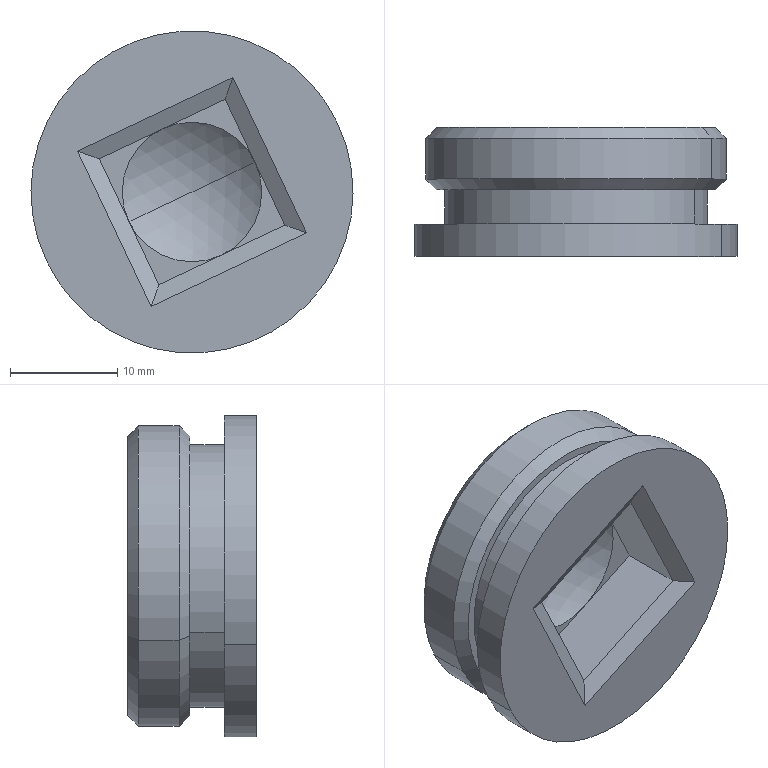Part | SolidWorks | features BaseBody 1 | 1 solid | 30 faces | box 30 x 12 x 30 mm | volume 5796 mm3 | plane 16 | cylinder 8 | cone 4 | sphere 2 | commonest cylinder face diameters 13 x2 24.5 x2 28 x2 30 x2
STEP:
#1=CARTESIAN_POINT('',(-57.117,-80.904,50.261));
#2=VERTEX_POINT('',#1);
#3=CARTESIAN_POINT('',(-31.809,-80.904,62.239));
#4=VERTEX_POINT('',#3);
#5=CARTESIAN_POINT('',(-44.463,-80.904,56.25));
#6=DIRECTION('',(0.,1.,0.));
#7=DIRECTION('',(0.9039,0.,0.4278));
#8=AXIS2_PLACEMENT_3D('',#5,#6,#7);
#9=CIRCLE('',#8,14.);
#10=EDGE_CURVE('',#2,#4,#9,.T.);
#11=ORIENTED_EDGE('',*,*,#10,.T.);
#12=CARTESIAN_POINT('',(-31.809,-77.104,62.239));
#13=VERTEX_POINT('',#12);
#14=CARTESIAN_POINT('',(-31.809,-81.904,62.239));
#15=DIRECTION('',(0.,1.,0.));
#16=VECTOR('',#15,1000.);
#17=LINE('',#14,#16);
#18=EDGE_CURVE('',#4,#13,#17,.T.);
#19=ORIENTED_EDGE('',*,*,#18,.T.);
#20=CARTESIAN_POINT('',(-57.117,-77.104,50.261));
#21=VERTEX_POINT('',#20);
#22=CARTESIAN_POINT('',(-44.463,-77.104,56.25));
#23=DIRECTION('',(0.,-1.,0.));
#24=DIRECTION('',(0.9039,0.,0.4278));
#25=AXIS2_PLACEMENT_3D('',#22,#23,#24);
#26=CIRCLE('',#25,14.);
#27=EDGE_CURVE('',#13,#21,#26,.T.);
#28=ORIENTED_EDGE('',*,*,#27,.T.);
#29=CARTESIAN_POINT('',(-57.117,-81.904,50.261));
#30=DIRECTION('',(0.,1.,0.));
#31=VECTOR('',#30,1000.);
#32=LINE('',#29,#31);
#33=EDGE_CURVE('',#2,#21,#32,.T.);
#34=ORIENTED_EDGE('',*,*,#33,.F.);
#35=EDGE_LOOP('',(#11,#19,#28,#34));
#36=FACE_OUTER_BOUND('',#35,.T.);
#37=CARTESIAN_POINT('',(-44.463,-81.904,56.25));
#38=DIRECTION('',(0.,1.,0.));
#39=DIRECTION('',(-0.9039,0.,-0.4278));
#40=AXIS2_PLACEMENT_3D('',#37,#38,#39);
#41=CYLINDRICAL_SURFACE('',#40,14.);
#42=ADVANCED_FACE('',(#36),#41,.T.);
#43=CARTESIAN_POINT('',(-33.39,-85.104,61.491));
#44=VERTEX_POINT('',#43);
#45=CARTESIAN_POINT('',(-55.535,-85.104,51.009));
#46=VERTEX_POINT('',#45);
#47=CARTESIAN_POINT('',(-44.463,-85.104,56.25));
#48=DIRECTION('',(0.,-1.,0.));
#49=DIRECTION('',(0.9039,0.,0.4278));
#50=AXIS2_PLACEMENT_3D('',#47,#48,#49);
#51=CIRCLE('',#50,12.25);
#52=EDGE_CURVE('',#44,#46,#51,.T.);
#53=ORIENTED_EDGE('',*,*,#52,.F.);
#54=CARTESIAN_POINT('',(-33.39,-81.904,61.491));
#55=VERTEX_POINT('',#54);
#56=CARTESIAN_POINT('',(-33.39,-85.104,61.491));
#57=DIRECTION('',(0.,1.,0.));
#58=VECTOR('',#57,1000.);
#59=LINE('',#56,#58);
#60=EDGE_CURVE('',#44,#55,#59,.T.);
#61=ORIENTED_EDGE('',*,*,#60,.T.);
#62=CARTESIAN_POINT('',(-55.535,-81.904,51.009));
#63=VERTEX_POINT('',#62);
#64=CARTESIAN_POINT('',(-44.463,-81.904,56.25));
#65=DIRECTION('',(0.,-1.,0.));
#66=DIRECTION('',(0.9039,0.,0.4278));
#67=AXIS2_PLACEMENT_3D('',#64,#65,#66);
#68=CIRCLE('',#67,12.25);
#69=EDGE_CURVE('',#55,#63,#68,.T.);
#70=ORIENTED_EDGE('',*,*,#69,.T.);
#71=CARTESIAN_POINT('',(-55.535,-85.104,51.009));
#72=DIRECTION('',(0.,1.,0.));
#73=VECTOR('',#72,1000.);
#74=LINE('',#71,#73);
#75=EDGE_CURVE('',#46,#63,#74,.T.);
#76=ORIENTED_EDGE('',*,*,#75,.F.);
#77=EDGE_LOOP('',(#53,#61,#70,#76));
#78=FACE_OUTER_BOUND('',#77,.T.);
#79=CARTESIAN_POINT('',(-44.463,-85.104,56.25));
#80=DIRECTION('',(0.,1.,0.));
#81=DIRECTION('',(-0.9039,0.,-0.4278));
#82=AXIS2_PLACEMENT_3D('',#79,#80,#81);
#83=CYLINDRICAL_SURFACE('',#82,12.25);
#84=ADVANCED_FACE('',(#78),#83,.T.);
#85=CARTESIAN_POINT('',(-30.905,-88.104,62.667));
#86=VERTEX_POINT('',#85);
#87=CARTESIAN_POINT('',(-58.021,-88.104,49.833));
#88=VERTEX_POINT('',#87);
#89=CARTESIAN_POINT('',(-44.463,-88.104,56.25));
#90=DIRECTION('',(0.,-1.,0.));
#91=DIRECTION('',(0.9039,0.,0.4278));
#92=AXIS2_PLACEMENT_3D('',#89,#90,#91);
#93=CIRCLE('',#92,15.);
#94=EDGE_CURVE('',#86,#88,#93,.T.);
#95=ORIENTED_EDGE('',*,*,#94,.F.);
#96=CARTESIAN_POINT('',(-30.905,-85.104,62.667));
#97=VERTEX_POINT('',#96);
#98=CARTESIAN_POINT('',(-30.905,-88.104,62.667));
#99=DIRECTION('',(0.,1.,0.));
#100=VECTOR('',#99,1000.);
#101=LINE('',#98,#100);
#102=EDGE_CURVE('',#86,#97,#101,.T.);
#103=ORIENTED_EDGE('',*,*,#102,.T.);
#104=CARTESIAN_POINT('',(-58.021,-85.104,49.833));
#105=VERTEX_POINT('',#104);
#106=CARTESIAN_POINT('',(-44.463,-85.104,56.25));
#107=DIRECTION('',(0.,-1.,0.));
#108=DIRECTION('',(0.9039,0.,0.4278));
#109=AXIS2_PLACEMENT_3D('',#106,#107,#108);
#110=CIRCLE('',#109,15.);
#111=EDGE_CURVE('',#97,#105,#110,.T.);
#112=ORIENTED_EDGE('',*,*,#111,.T.);
#113=CARTESIAN_POINT('',(-58.021,-88.104,49.833));
#114=DIRECTION('',(0.,1.,0.));
#115=VECTOR('',#114,1000.);
#116=LINE('',#113,#115);
#117=EDGE_CURVE('',#88,#105,#116,.T.);
#118=ORIENTED_EDGE('',*,*,#117,.F.);
#119=EDGE_LOOP('',(#95,#103,#112,#118));
#120=FACE_OUTER_BOUND('',#119,.T.);
#121=CARTESIAN_POINT('',(-44.463,-88.104,56.25));
#122=DIRECTION('',(0.,1.,0.));
#123=DIRECTION('',(-0.9039,0.,-0.4278));
#124=AXIS2_PLACEMENT_3D('',#121,#122,#123);
#125=CYLINDRICAL_SURFACE('',#124,15.);
#126=ADVANCED_FACE('',(#120),#125,.T.);
#127=CARTESIAN_POINT('',(-50.338,-81.504,53.469));
#128=VERTEX_POINT('',#127);
#129=CARTESIAN_POINT('',(-38.588,-81.504,59.031));
#130=VERTEX_POINT('',#129);
#131=CARTESIAN_POINT('',(-44.463,-81.504,56.25));
#132=DIRECTION('',(0.,1.,0.));
#133=DIRECTION('',(-0.9039,0.,-0.4278));
#134=AXIS2_PLACEMENT_3D('',#131,#132,#133);
#135=CIRCLE('',#134,6.5);
#136=EDGE_CURVE('',#128,#130,#135,.T.);
#137=ORIENTED_EDGE('',*,*,#136,.F.);
#138=CARTESIAN_POINT('',(-44.463,-79.104,56.25));
#139=VERTEX_POINT('',#138);
#140=CARTESIAN_POINT('',(-44.463,-89.104,56.25));
#141=DIRECTION('',(0.4278,0.,-0.9039));
#142=DIRECTION('',(-0.9039,0.,-0.4278));
#143=AXIS2_PLACEMENT_3D('',#140,#141,#142);
#144=CIRCLE('',#143,10.);
#145=EDGE_CURVE('',#128,#139,#144,.T.);
#146=ORIENTED_EDGE('',*,*,#145,.T.);
#147=CARTESIAN_POINT('',(-44.463,-89.104,56.25));
#148=DIRECTION('',(-0.4278,0.,0.9039));
#149=DIRECTION('',(0.9039,0.,0.4278));
#150=AXIS2_PLACEMENT_3D('',#147,#148,#149);
#151=CIRCLE('',#150,10.);
#152=EDGE_CURVE('',#130,#139,#151,.T.);
#153=ORIENTED_EDGE('',*,*,#152,.F.);
#154=EDGE_LOOP('',(#137,#146,#153));
#155=FACE_OUTER_BOUND('',#154,.T.);
#156=CARTESIAN_POINT('',(-44.463,-89.104,56.25));
#157=DIRECTION('',(0.4278,0.,-0.9039));
#158=DIRECTION('',(0.9039,0.,0.4278));
#159=AXIS2_PLACEMENT_3D('',#156,#157,#158);
#160=SPHERICAL_SURFACE('',#159,10.);
#161=ADVANCED_FACE('',(#155),#160,.F.);
#162=CARTESIAN_POINT('',(-41.682,-81.505,50.375));
#163=VERTEX_POINT('',#162);
#164=CARTESIAN_POINT('',(-38.588,-81.505,59.031));
#165=VERTEX_POINT('',#164);
#166=CARTESIAN_POINT('',(-44.463,-81.505,56.25));
#167=DIRECTION('',(0.,-1.,0.));
#168=DIRECTION('',(0.9039,0.,0.4278));
#169=AXIS2_PLACEMENT_3D('',#166,#167,#168);
#170=CIRCLE('',#169,6.5);
#171=EDGE_CURVE('',#163,#165,#170,.T.);
#172=ORIENTED_EDGE('',*,*,#171,.T.);
#173=CARTESIAN_POINT('',(-38.588,-79.104,59.031));
#174=DIRECTION('',(0.,1.,0.));
#175=VECTOR('',#174,1000.);
#176=LINE('',#173,#175);
#177=EDGE_CURVE('',#165,#130,#176,.T.);
#178=ORIENTED_EDGE('',*,*,#177,.T.);
#179=CARTESIAN_POINT('',(-44.463,-81.504,56.25));
#180=DIRECTION('',(0.,1.,0.));
#181=DIRECTION('',(-0.9039,0.,-0.4278));
#182=AXIS2_PLACEMENT_3D('',#179,#180,#181);
#183=CIRCLE('',#182,6.5);
#184=EDGE_CURVE('',#130,#128,#183,.T.);
#185=ORIENTED_EDGE('',*,*,#184,.T.);
#186=CARTESIAN_POINT('',(-50.338,-81.505,53.469));
#187=VERTEX_POINT('',#186);
#188=CARTESIAN_POINT('',(-50.338,-79.104,53.469));
#189=DIRECTION('',(0.,1.,0.));
#190=VECTOR('',#189,1000.);
#191=LINE('',#188,#190);
#192=EDGE_CURVE('',#187,#128,#191,.T.);
#193=ORIENTED_EDGE('',*,*,#192,.F.);
#194=CARTESIAN_POINT('',(-44.463,-81.505,56.25));
#195=DIRECTION('',(0.,-1.,0.));
#196=DIRECTION('',(0.9039,0.,0.4278));
#197=AXIS2_PLACEMENT_3D('',#194,#195,#196);
#198=CIRCLE('',#197,6.5);
#199=EDGE_CURVE('',#187,#163,#198,.T.);
#200=ORIENTED_EDGE('',*,*,#199,.T.);
#201=EDGE_LOOP('',(#172,#178,#185,#193,#200));
#202=FACE_OUTER_BOUND('',#201,.T.);
#203=CARTESIAN_POINT('',(-44.463,-79.104,56.25));
#204=DIRECTION('',(0.,1.,0.));
#205=DIRECTION('',(-0.9039,0.,-0.4278));
#206=AXIS2_PLACEMENT_3D('',#203,#204,#205);
#207=CYLINDRICAL_SURFACE('',#206,6.5);
#208=ADVANCED_FACE('',(#202),#207,.F.);
#209=CARTESIAN_POINT('',(-56.213,-76.104,50.689));
#210=VERTEX_POINT('',#209);
#211=CARTESIAN_POINT('',(-32.713,-76.104,61.811));
#212=VERTEX_POINT('',#211);
#213=CARTESIAN_POINT('',(-44.463,-76.104,56.25));
#214=DIRECTION('',(0.,1.,0.));
#215=DIRECTION('',(0.9039,0.,0.4278));
#216=AXIS2_PLACEMENT_3D('',#213,#214,#215);
#217=CIRCLE('',#216,13.);
#218=EDGE_CURVE('',#210,#212,#217,.T.);
#219=ORIENTED_EDGE('',*,*,#218,.F.);
#220=CARTESIAN_POINT('',(-57.117,-77.104,50.261));
#221=DIRECTION('',(-0.6391,-0.7071,-0.3025));
#222=VECTOR('',#221,1000.);
#223=LINE('',#220,#222);
#224=EDGE_CURVE('',#210,#21,#223,.T.);
#225=ORIENTED_EDGE('',*,*,#224,.T.);
#226=ORIENTED_EDGE('',*,*,#27,.F.);
#227=CARTESIAN_POINT('',(-31.809,-77.104,62.239));
#228=DIRECTION('',(0.6391,-0.7071,0.3025));
#229=VECTOR('',#228,1000.);
#230=LINE('',#227,#229);
#231=EDGE_CURVE('',#212,#13,#230,.T.);
#232=ORIENTED_EDGE('',*,*,#231,.F.);
#233=EDGE_LOOP('',(#219,#225,#226,#232));
#234=FACE_OUTER_BOUND('',#233,.T.);
#235=CARTESIAN_POINT('',(-44.463,-77.104,56.25));
#236=DIRECTION('',(0.,-1.,0.));
#237=DIRECTION('',(0.9039,0.,0.4278));
#238=AXIS2_PLACEMENT_3D('',#235,#236,#237);
#239=CONICAL_SURFACE('',#238,14.,0.7854);
#240=ADVANCED_FACE('',(#234),#239,.T.);
#241=CARTESIAN_POINT('',(-32.713,-81.904,61.811));
#242=VERTEX_POINT('',#241);
#243=CARTESIAN_POINT('',(-56.213,-81.904,50.689));
#244=VERTEX_POINT('',#243);
#245=CARTESIAN_POINT('',(-44.463,-81.904,56.25));
#246=DIRECTION('',(0.,-1.,0.));
#247=DIRECTION('',(0.9039,0.,0.4278));
#248=AXIS2_PLACEMENT_3D('',#245,#246,#247);
#249=CIRCLE('',#248,13.);
#250=EDGE_CURVE('',#242,#244,#249,.T.);
#251=ORIENTED_EDGE('',*,*,#250,.F.);
#252=CARTESIAN_POINT('',(-32.713,-81.904,61.811));
#253=DIRECTION('',(0.6391,0.7071,0.3025));
#254=VECTOR('',#253,1000.);
#255=LINE('',#252,#254);
#256=EDGE_CURVE('',#242,#4,#255,.T.);
#257=ORIENTED_EDGE('',*,*,#256,.T.);
#258=ORIENTED_EDGE('',*,*,#10,.F.);
#259=CARTESIAN_POINT('',(-56.213,-81.904,50.689));
#260=DIRECTION('',(-0.6391,0.7071,-0.3025));
#261=VECTOR('',#260,1000.);
#262=LINE('',#259,#261);
#263=EDGE_CURVE('',#244,#2,#262,.T.);
#264=ORIENTED_EDGE('',*,*,#263,.F.);
#265=EDGE_LOOP('',(#251,#257,#258,#264));
#266=FACE_OUTER_BOUND('',#265,.T.);
#267=CARTESIAN_POINT('',(-44.463,-81.904,56.25));
#268=DIRECTION('',(0.,1.,0.));
#269=DIRECTION('',(-0.9039,0.,-0.4278));
#270=AXIS2_PLACEMENT_3D('',#267,#268,#269);
#271=CONICAL_SURFACE('',#270,13.,0.7854);
#272=ADVANCED_FACE('',(#266),#271,.T.);
#273=CARTESIAN_POINT('',(-53.119,-87.238,59.344));
#274=VERTEX_POINT('',#273);
#275=CARTESIAN_POINT('',(-55.116,-88.104,60.059));
#276=VERTEX_POINT('',#275);
#277=CARTESIAN_POINT('',(-53.119,-87.238,59.344));
#278=DIRECTION('',(-0.8718,-0.378,0.3117));
#279=VECTOR('',#278,1000.);
#280=LINE('',#277,#279);
#281=EDGE_CURVE('',#274,#276,#280,.T.);
#282=ORIENTED_EDGE('',*,*,#281,.T.);
#283=CARTESIAN_POINT('',(-48.271,-88.104,45.597));
#284=VERTEX_POINT('',#283);
#285=CARTESIAN_POINT('',(-54.475,-88.104,58.703));
#286=DIRECTION('',(-0.4278,0.,0.9039));
#287=VECTOR('',#286,1000.);
#288=LINE('',#285,#287);
#289=EDGE_CURVE('',#284,#276,#288,.T.);
#290=ORIENTED_EDGE('',*,*,#289,.F.);
#291=CARTESIAN_POINT('',(-47.557,-87.238,47.594));
#292=VERTEX_POINT('',#291);
#293=CARTESIAN_POINT('',(-44.905,-84.021,55.013));
#294=DIRECTION('',(0.3117,0.378,0.8718));
#295=VECTOR('',#294,1000.);
#296=LINE('',#293,#295);
#297=EDGE_CURVE('',#284,#292,#296,.T.);
#298=ORIENTED_EDGE('',*,*,#297,.T.);
#299=CARTESIAN_POINT('',(-47.557,-87.238,47.594));
#300=DIRECTION('',(0.4278,0.,-0.9039));
#301=VECTOR('',#300,1000.);
#302=LINE('',#299,#301);
#303=EDGE_CURVE('',#274,#292,#302,.T.);
#304=ORIENTED_EDGE('',*,*,#303,.F.);
#305=EDGE_LOOP('',(#282,#290,#298,#304));
#306=FACE_OUTER_BOUND('',#305,.T.);
#307=CARTESIAN_POINT('',(-53.119,-87.238,59.344));
#308=DIRECTION('',(0.4519,-0.866,0.2139));
#309=DIRECTION('',(0.,-0.2398,-0.9708));
#310=AXIS2_PLACEMENT_3D('',#307,#308,#309);
#311=PLANE('',#310);
#312=ADVANCED_FACE('',(#306),#311,.T.);
#313=CARTESIAN_POINT('',(-33.809,-88.104,52.441));
#314=VERTEX_POINT('',#313);
#315=CARTESIAN_POINT('',(-35.807,-87.238,53.156));
#316=VERTEX_POINT('',#315);
#317=CARTESIAN_POINT('',(-43.226,-84.021,55.808));
#318=DIRECTION('',(-0.8718,0.378,0.3117));
#319=VECTOR('',#318,1000.);
#320=LINE('',#317,#319);
#321=EDGE_CURVE('',#314,#316,#320,.T.);
#322=ORIENTED_EDGE('',*,*,#321,.T.);
#323=CARTESIAN_POINT('',(-35.807,-87.238,53.156));
#324=DIRECTION('',(0.9039,0.,0.4278));
#325=VECTOR('',#324,1000.);
#326=LINE('',#323,#325);
#327=EDGE_CURVE('',#292,#316,#326,.T.);
#328=ORIENTED_EDGE('',*,*,#327,.F.);
#329=ORIENTED_EDGE('',*,*,#297,.F.);
#330=CARTESIAN_POINT('',(-46.916,-88.104,46.238));
#331=DIRECTION('',(-0.9039,0.,-0.4278));
#332=VECTOR('',#331,1000.);
#333=LINE('',#330,#332);
#334=EDGE_CURVE('',#314,#284,#333,.T.);
#335=ORIENTED_EDGE('',*,*,#334,.F.);
#336=EDGE_LOOP('',(#322,#328,#329,#335));
#337=FACE_OUTER_BOUND('',#336,.T.);
#338=CARTESIAN_POINT('',(-47.557,-87.238,47.594));
#339=DIRECTION('',(-0.2139,-0.866,0.4519));
#340=DIRECTION('',(-0.9708,0.2398,0.));
#341=AXIS2_PLACEMENT_3D('',#338,#339,#340);
#342=PLANE('',#341);
#343=ADVANCED_FACE('',(#337),#342,.T.);
#344=CARTESIAN_POINT('',(-41.368,-87.238,64.906));
#345=VERTEX_POINT('',#344);
#346=CARTESIAN_POINT('',(-40.654,-88.104,66.903));
#347=VERTEX_POINT('',#346);
#348=CARTESIAN_POINT('',(-44.021,-84.021,57.487));
#349=DIRECTION('',(0.3117,-0.378,0.8718));
#350=VECTOR('',#349,1000.);
#351=LINE('',#348,#350);
#352=EDGE_CURVE('',#345,#347,#351,.T.);
#353=ORIENTED_EDGE('',*,*,#352,.T.);
#354=CARTESIAN_POINT('',(-42.01,-88.104,66.262));
#355=DIRECTION('',(0.9039,0.,0.4278));
#356=VECTOR('',#355,1000.);
#357=LINE('',#354,#356);
#358=EDGE_CURVE('',#276,#347,#357,.T.);
#359=ORIENTED_EDGE('',*,*,#358,.F.);
#360=ORIENTED_EDGE('',*,*,#281,.F.);
#361=CARTESIAN_POINT('',(-53.119,-87.238,59.344));
#362=DIRECTION('',(-0.9039,0.,-0.4278));
#363=VECTOR('',#362,1000.);
#364=LINE('',#361,#363);
#365=EDGE_CURVE('',#345,#274,#364,.T.);
#366=ORIENTED_EDGE('',*,*,#365,.F.);
#367=EDGE_LOOP('',(#353,#359,#360,#366));
#368=FACE_OUTER_BOUND('',#367,.T.);
#369=CARTESIAN_POINT('',(-53.119,-87.238,59.344));
#370=DIRECTION('',(0.2139,-0.866,-0.4519));
#371=DIRECTION('',(0.,0.4626,-0.8865));
#372=AXIS2_PLACEMENT_3D('',#369,#370,#371);
#373=PLANE('',#372);
#374=ADVANCED_FACE('',(#368),#373,.T.);
#375=ORIENTED_EDGE('',*,*,#321,.F.);
#376=CARTESIAN_POINT('',(-34.451,-88.104,53.797));
#377=DIRECTION('',(0.4278,0.,-0.9039));
#378=VECTOR('',#377,1000.);
#379=LINE('',#376,#378);
#380=EDGE_CURVE('',#347,#314,#379,.T.);
#381=ORIENTED_EDGE('',*,*,#380,.F.);
#382=ORIENTED_EDGE('',*,*,#352,.F.);
#383=CARTESIAN_POINT('',(-41.368,-87.238,64.906));
#384=DIRECTION('',(-0.4278,0.,0.9039));
#385=VECTOR('',#384,1000.);
#386=LINE('',#383,#385);
#387=EDGE_CURVE('',#316,#345,#386,.T.);
#388=ORIENTED_EDGE('',*,*,#387,.F.);
#389=EDGE_LOOP('',(#375,#381,#382,#388));
#390=FACE_OUTER_BOUND('',#389,.T.);
#391=CARTESIAN_POINT('',(-41.368,-87.238,64.906));
#392=DIRECTION('',(-0.4519,-0.866,-0.2139));
#393=DIRECTION('',(-0.8865,0.4626,0.));
#394=AXIS2_PLACEMENT_3D('',#391,#392,#393);
#395=PLANE('',#394);
#396=ADVANCED_FACE('',(#390),#395,.T.);
#397=ORIENTED_EDGE('',*,*,#256,.F.);
#398=CARTESIAN_POINT('',(-44.463,-81.904,56.25));
#399=DIRECTION('',(0.,-1.,0.));
#400=DIRECTION('',(0.9039,0.,0.4278));
#401=AXIS2_PLACEMENT_3D('',#398,#399,#400);
#402=CIRCLE('',#401,13.);
#403=EDGE_CURVE('',#244,#242,#402,.T.);
#404=ORIENTED_EDGE('',*,*,#403,.F.);
#405=ORIENTED_EDGE('',*,*,#263,.T.);
#406=CARTESIAN_POINT('',(-44.463,-80.904,56.25));
#407=DIRECTION('',(0.,1.,0.));
#408=DIRECTION('',(0.9039,0.,0.4278));
#409=AXIS2_PLACEMENT_3D('',#406,#407,#408);
#410=CIRCLE('',#409,14.);
#411=EDGE_CURVE('',#4,#2,#410,.T.);
#412=ORIENTED_EDGE('',*,*,#411,.F.);
#413=EDGE_LOOP('',(#397,#404,#405,#412));
#414=FACE_OUTER_BOUND('',#413,.T.);
#415=CARTESIAN_POINT('',(-44.463,-81.904,56.25));
#416=DIRECTION('',(0.,1.,0.));
#417=DIRECTION('',(-0.9039,0.,-0.4278));
#418=AXIS2_PLACEMENT_3D('',#415,#416,#417);
#419=CONICAL_SURFACE('',#418,13.,0.7854);
#420=ADVANCED_FACE('',(#414),#419,.T.);
#421=ORIENTED_EDGE('',*,*,#224,.F.);
#422=CARTESIAN_POINT('',(-44.463,-76.104,56.25));
#423=DIRECTION('',(0.,1.,0.));
#424=DIRECTION('',(0.9039,0.,0.4278));
#425=AXIS2_PLACEMENT_3D('',#422,#423,#424);
#426=CIRCLE('',#425,13.);
#427=EDGE_CURVE('',#212,#210,#426,.T.);
#428=ORIENTED_EDGE('',*,*,#427,.F.);
#429=ORIENTED_EDGE('',*,*,#231,.T.);
#430=CARTESIAN_POINT('',(-44.463,-77.104,56.25));
#431=DIRECTION('',(0.,-1.,0.));
#432=DIRECTION('',(0.9039,0.,0.4278));
#433=AXIS2_PLACEMENT_3D('',#430,#431,#432);
#434=CIRCLE('',#433,14.);
#435=EDGE_CURVE('',#21,#13,#434,.T.);
#436=ORIENTED_EDGE('',*,*,#435,.F.);
#437=EDGE_LOOP('',(#421,#428,#429,#436));
#438=FACE_OUTER_BOUND('',#437,.T.);
#439=CARTESIAN_POINT('',(-44.463,-77.104,56.25));
#440=DIRECTION('',(0.,-1.,0.));
#441=DIRECTION('',(0.9039,0.,0.4278));
#442=AXIS2_PLACEMENT_3D('',#439,#440,#441);
#443=CONICAL_SURFACE('',#442,14.,0.7854);
#444=ADVANCED_FACE('',(#438),#443,.T.);
#445=ORIENTED_EDGE('',*,*,#177,.F.);
#446=CARTESIAN_POINT('',(-47.244,-81.505,62.125));
#447=VERTEX_POINT('',#446);
#448=CARTESIAN_POINT('',(-44.463,-81.505,56.25));
#449=DIRECTION('',(0.,-1.,0.));
#450=DIRECTION('',(0.9039,0.,0.4278));
#451=AXIS2_PLACEMENT_3D('',#448,#449,#450);
#452=CIRCLE('',#451,6.5);
#453=EDGE_CURVE('',#165,#447,#452,.T.);
#454=ORIENTED_EDGE('',*,*,#453,.T.);
#455=CARTESIAN_POINT('',(-44.463,-81.505,56.25));
#456=DIRECTION('',(0.,-1.,0.));
#457=DIRECTION('',(0.9039,0.,0.4278));
#458=AXIS2_PLACEMENT_3D('',#455,#456,#457);
#459=CIRCLE('',#458,6.5);
#460=EDGE_CURVE('',#447,#187,#459,.T.);
#461=ORIENTED_EDGE('',*,*,#460,.T.);
#462=ORIENTED_EDGE('',*,*,#192,.T.);
#463=ORIENTED_EDGE('',*,*,#136,.T.);
#464=EDGE_LOOP('',(#445,#454,#461,#462,#463));
#465=FACE_OUTER_BOUND('',#464,.T.);
#466=CARTESIAN_POINT('',(-44.463,-79.104,56.25));
#467=DIRECTION('',(0.,1.,0.));
#468=DIRECTION('',(-0.9039,0.,-0.4278));
#469=AXIS2_PLACEMENT_3D('',#466,#467,#468);
#470=CYLINDRICAL_SURFACE('',#469,6.5);
#471=ADVANCED_FACE('',(#465),#470,.F.);
#472=ORIENTED_EDGE('',*,*,#145,.F.);
#473=ORIENTED_EDGE('',*,*,#184,.F.);
#474=ORIENTED_EDGE('',*,*,#152,.T.);
#475=EDGE_LOOP('',(#472,#473,#474));
#476=FACE_OUTER_BOUND('',#475,.T.);
#477=CARTESIAN_POINT('',(-44.463,-89.104,56.25));
#478=DIRECTION('',(0.4278,0.,-0.9039));
#479=DIRECTION('',(0.9039,0.,0.4278));
#480=AXIS2_PLACEMENT_3D('',#477,#478,#479);
#481=SPHERICAL_SURFACE('',#480,10.);
#482=ADVANCED_FACE('',(#476),#481,.F.);
#483=CARTESIAN_POINT('',(-35.807,-81.505,53.156));
#484=VERTEX_POINT('',#483);
#485=CARTESIAN_POINT('',(-47.557,-81.505,47.594));
#486=DIRECTION('',(0.9039,0.,0.4278));
#487=VECTOR('',#486,1000.);
#488=LINE('',#485,#487);
#489=EDGE_CURVE('',#163,#484,#488,.T.);
#490=ORIENTED_EDGE('',*,*,#489,.T.);
#491=CARTESIAN_POINT('',(-41.368,-81.505,64.906));
#492=DIRECTION('',(-0.4278,0.,0.9039));
#493=VECTOR('',#492,1000.);
#494=LINE('',#491,#493);
#495=EDGE_CURVE('',#484,#165,#494,.T.);
#496=ORIENTED_EDGE('',*,*,#495,.T.);
#497=ORIENTED_EDGE('',*,*,#171,.F.);
#498=EDGE_LOOP('',(#490,#496,#497));
#499=FACE_OUTER_BOUND('',#498,.T.);
#500=CARTESIAN_POINT('',(-47.557,-81.505,47.594));
#501=DIRECTION('',(0.,-1.,0.));
#502=DIRECTION('',(-1.,0.,0.));
#503=AXIS2_PLACEMENT_3D('',#500,#501,#502);
#504=PLANE('',#503);
#505=ADVANCED_FACE('',(#499),#504,.T.);
#506=CARTESIAN_POINT('',(-47.557,-81.505,47.594));
#507=VERTEX_POINT('',#506);
#508=CARTESIAN_POINT('',(-53.119,-81.505,59.344));
#509=DIRECTION('',(0.4278,0.,-0.9039));
#510=VECTOR('',#509,1000.);
#511=LINE('',#508,#510);
#512=EDGE_CURVE('',#187,#507,#511,.T.);
#513=ORIENTED_EDGE('',*,*,#512,.T.);
#514=CARTESIAN_POINT('',(-47.557,-81.505,47.594));
#515=DIRECTION('',(0.9039,0.,0.4278));
#516=VECTOR('',#515,1000.);
#517=LINE('',#514,#516);
#518=EDGE_CURVE('',#507,#163,#517,.T.);
#519=ORIENTED_EDGE('',*,*,#518,.T.);
#520=ORIENTED_EDGE('',*,*,#199,.F.);
#521=EDGE_LOOP('',(#513,#519,#520));
#522=FACE_OUTER_BOUND('',#521,.T.);
#523=CARTESIAN_POINT('',(-47.557,-81.505,47.594));
#524=DIRECTION('',(0.,-1.,0.));
#525=DIRECTION('',(-1.,0.,0.));
#526=AXIS2_PLACEMENT_3D('',#523,#524,#525);
#527=PLANE('',#526);
#528=ADVANCED_FACE('',(#522),#527,.T.);
#529=CARTESIAN_POINT('',(-53.119,-81.505,59.344));
#530=VERTEX_POINT('',#529);
#531=CARTESIAN_POINT('',(-53.119,-81.505,59.344));
#532=DIRECTION('',(-0.9039,0.,-0.4278));
#533=VECTOR('',#532,1000.);
#534=LINE('',#531,#533);
#535=EDGE_CURVE('',#447,#530,#534,.T.);
#536=ORIENTED_EDGE('',*,*,#535,.T.);
#537=CARTESIAN_POINT('',(-53.119,-81.505,59.344));
#538=DIRECTION('',(0.4278,0.,-0.9039));
#539=VECTOR('',#538,1000.);
#540=LINE('',#537,#539);
#541=EDGE_CURVE('',#530,#187,#540,.T.);
#542=ORIENTED_EDGE('',*,*,#541,.T.);
#543=ORIENTED_EDGE('',*,*,#460,.F.);
#544=EDGE_LOOP('',(#536,#542,#543));
#545=FACE_OUTER_BOUND('',#544,.T.);
#546=CARTESIAN_POINT('',(-47.557,-81.505,47.594));
#547=DIRECTION('',(0.,-1.,0.));
#548=DIRECTION('',(-1.,0.,0.));
#549=AXIS2_PLACEMENT_3D('',#546,#547,#548);
#550=PLANE('',#549);
#551=ADVANCED_FACE('',(#545),#550,.T.);
#552=CARTESIAN_POINT('',(-41.368,-81.505,64.906));
#553=VERTEX_POINT('',#552);
#554=CARTESIAN_POINT('',(-41.368,-81.505,64.906));
#555=DIRECTION('',(-0.4278,0.,0.9039));
#556=VECTOR('',#555,1000.);
#557=LINE('',#554,#556);
#558=EDGE_CURVE('',#165,#553,#557,.T.);
#559=ORIENTED_EDGE('',*,*,#558,.T.);
#560=CARTESIAN_POINT('',(-53.119,-81.505,59.344));
#561=DIRECTION('',(-0.9039,0.,-0.4278));
#562=VECTOR('',#561,1000.);
#563=LINE('',#560,#562);
#564=EDGE_CURVE('',#553,#447,#563,.T.);
#565=ORIENTED_EDGE('',*,*,#564,.T.);
#566=ORIENTED_EDGE('',*,*,#453,.F.);
#567=EDGE_LOOP('',(#559,#565,#566));
#568=FACE_OUTER_BOUND('',#567,.T.);
#569=CARTESIAN_POINT('',(-47.557,-81.505,47.594));
#570=DIRECTION('',(0.,-1.,0.));
#571=DIRECTION('',(-1.,0.,0.));
#572=AXIS2_PLACEMENT_3D('',#569,#570,#571);
#573=PLANE('',#572);
#574=ADVANCED_FACE('',(#568),#573,.T.);
#575=CARTESIAN_POINT('',(-47.557,-81.505,47.594));
#576=DIRECTION('',(0.,-1.,0.));
#577=VECTOR('',#576,1000.);
#578=LINE('',#575,#577);
#579=EDGE_CURVE('',#507,#292,#578,.T.);
#580=ORIENTED_EDGE('',*,*,#579,.T.);
#581=ORIENTED_EDGE('',*,*,#327,.T.);
#582=CARTESIAN_POINT('',(-35.807,-81.505,53.156));
#583=DIRECTION('',(0.,-1.,0.));
#584=VECTOR('',#583,1000.);
#585=LINE('',#582,#584);
#586=EDGE_CURVE('',#484,#316,#585,.T.);
#587=ORIENTED_EDGE('',*,*,#586,.F.);
#588=ORIENTED_EDGE('',*,*,#489,.F.);
#589=ORIENTED_EDGE('',*,*,#518,.F.);
#590=EDGE_LOOP('',(#580,#581,#587,#588,#589));
#591=FACE_OUTER_BOUND('',#590,.T.);
#592=CARTESIAN_POINT('',(-47.557,-81.505,47.594));
#593=DIRECTION('',(0.4278,0.,-0.9039));
#594=DIRECTION('',(0.,-1.,0.));
#595=AXIS2_PLACEMENT_3D('',#592,#593,#594);
#596=PLANE('',#595);
#597=ADVANCED_FACE('',(#591),#596,.F.);
#598=ORIENTED_EDGE('',*,*,#586,.T.);
#599=ORIENTED_EDGE('',*,*,#387,.T.);
#600=CARTESIAN_POINT('',(-41.368,-81.505,64.906));
#601=DIRECTION('',(0.,-1.,0.));
#602=VECTOR('',#601,1000.);
#603=LINE('',#600,#602);
#604=EDGE_CURVE('',#553,#345,#603,.T.);
#605=ORIENTED_EDGE('',*,*,#604,.F.);
#606=ORIENTED_EDGE('',*,*,#558,.F.);
#607=ORIENTED_EDGE('',*,*,#495,.F.);
#608=EDGE_LOOP('',(#598,#599,#605,#606,#607));
#609=FACE_OUTER_BOUND('',#608,.T.);
#610=CARTESIAN_POINT('',(-41.368,-81.505,64.906));
#611=DIRECTION('',(0.9039,0.,0.4278));
#612=DIRECTION('',(0.,-1.,0.));
#613=AXIS2_PLACEMENT_3D('',#610,#611,#612);
#614=PLANE('',#613);
#615=ADVANCED_FACE('',(#609),#614,.F.);
#616=ORIENTED_EDGE('',*,*,#604,.T.);
#617=ORIENTED_EDGE('',*,*,#365,.T.);
#618=CARTESIAN_POINT('',(-53.119,-81.505,59.344));
#619=DIRECTION('',(0.,-1.,0.));
#620=VECTOR('',#619,1000.);
#621=LINE('',#618,#620);
#622=EDGE_CURVE('',#530,#274,#621,.T.);
#623=ORIENTED_EDGE('',*,*,#622,.F.);
#624=ORIENTED_EDGE('',*,*,#535,.F.);
#625=ORIENTED_EDGE('',*,*,#564,.F.);
#626=EDGE_LOOP('',(#616,#617,#623,#624,#625));
#627=FACE_OUTER_BOUND('',#626,.T.);
#628=CARTESIAN_POINT('',(-53.119,-81.505,59.344));
#629=DIRECTION('',(-0.4278,0.,0.9039));
#630=DIRECTION('',(0.,1.,0.));
#631=AXIS2_PLACEMENT_3D('',#628,#629,#630);
#632=PLANE('',#631);
#633=ADVANCED_FACE('',(#627),#632,.F.);
#634=ORIENTED_EDGE('',*,*,#622,.T.);
#635=ORIENTED_EDGE('',*,*,#303,.T.);
#636=ORIENTED_EDGE('',*,*,#579,.F.);
#637=ORIENTED_EDGE('',*,*,#512,.F.);
#638=ORIENTED_EDGE('',*,*,#541,.F.);
#639=EDGE_LOOP('',(#634,#635,#636,#637,#638));
#640=FACE_OUTER_BOUND('',#639,.T.);
#641=CARTESIAN_POINT('',(-53.119,-81.505,59.344));
#642=DIRECTION('',(-0.9039,0.,-0.4278));
#643=DIRECTION('',(-0.4278,0.,0.9039));
#644=AXIS2_PLACEMENT_3D('',#641,#642,#643);
#645=PLANE('',#644);
#646=ADVANCED_FACE('',(#640),#645,.F.);
#647=ORIENTED_EDGE('',*,*,#102,.F.);
#648=CARTESIAN_POINT('',(-44.463,-88.104,56.25));
#649=DIRECTION('',(0.,-1.,0.));
#650=DIRECTION('',(0.9039,0.,0.4278));
#651=AXIS2_PLACEMENT_3D('',#648,#649,#650);
#652=CIRCLE('',#651,15.);
#653=EDGE_CURVE('',#88,#86,#652,.T.);
#654=ORIENTED_EDGE('',*,*,#653,.F.);
#655=ORIENTED_EDGE('',*,*,#117,.T.);
#656=CARTESIAN_POINT('',(-44.463,-85.104,56.25));
#657=DIRECTION('',(0.,-1.,0.));
#658=DIRECTION('',(0.9039,0.,0.4278));
#659=AXIS2_PLACEMENT_3D('',#656,#657,#658);
#660=CIRCLE('',#659,15.);
#661=EDGE_CURVE('',#105,#97,#660,.T.);
#662=ORIENTED_EDGE('',*,*,#661,.T.);
#663=EDGE_LOOP('',(#647,#654,#655,#662));
#664=FACE_OUTER_BOUND('',#663,.T.);
#665=CARTESIAN_POINT('',(-44.463,-88.104,56.25));
#666=DIRECTION('',(0.,1.,0.));
#667=DIRECTION('',(-0.9039,0.,-0.4278));
#668=AXIS2_PLACEMENT_3D('',#665,#666,#667);
#669=CYLINDRICAL_SURFACE('',#668,15.);
#670=ADVANCED_FACE('',(#664),#669,.T.);
#671=CARTESIAN_POINT('',(-44.463,-85.104,56.25));
#672=DIRECTION('',(0.,-1.,0.));
#673=DIRECTION('',(0.9039,0.,0.4278));
#674=AXIS2_PLACEMENT_3D('',#671,#672,#673);
#675=CIRCLE('',#674,12.25);
#676=EDGE_CURVE('',#46,#44,#675,.T.);
#677=ORIENTED_EDGE('',*,*,#676,.T.);
#678=ORIENTED_EDGE('',*,*,#52,.T.);
#679=EDGE_LOOP('',(#677,#678));
#680=FACE_BOUND('',#679,.T.);
#681=ORIENTED_EDGE('',*,*,#661,.F.);
#682=ORIENTED_EDGE('',*,*,#111,.F.);
#683=EDGE_LOOP('',(#681,#682));
#684=FACE_OUTER_BOUND('',#683,.T.);
#685=CARTESIAN_POINT('',(-44.463,-85.104,56.25));
#686=DIRECTION('',(0.,-1.,0.));
#687=DIRECTION('',(-1.,0.,0.));
#688=AXIS2_PLACEMENT_3D('',#685,#686,#687);
#689=PLANE('',#688);
#690=ADVANCED_FACE('',(#680,#684),#689,.F.);
#691=ORIENTED_EDGE('',*,*,#60,.F.);
#692=ORIENTED_EDGE('',*,*,#676,.F.);
#693=ORIENTED_EDGE('',*,*,#75,.T.);
#694=CARTESIAN_POINT('',(-44.463,-81.904,56.25));
#695=DIRECTION('',(0.,-1.,0.));
#696=DIRECTION('',(0.9039,0.,0.4278));
#697=AXIS2_PLACEMENT_3D('',#694,#695,#696);
#698=CIRCLE('',#697,12.25);
#699=EDGE_CURVE('',#63,#55,#698,.T.);
#700=ORIENTED_EDGE('',*,*,#699,.T.);
#701=EDGE_LOOP('',(#691,#692,#693,#700));
#702=FACE_OUTER_BOUND('',#701,.T.);
#703=CARTESIAN_POINT('',(-44.463,-85.104,56.25));
#704=DIRECTION('',(0.,1.,0.));
#705=DIRECTION('',(-0.9039,0.,-0.4278));
#706=AXIS2_PLACEMENT_3D('',#703,#704,#705);
#707=CYLINDRICAL_SURFACE('',#706,12.25);
#708=ADVANCED_FACE('',(#702),#707,.T.);
#709=ORIENTED_EDGE('',*,*,#427,.T.);
#710=ORIENTED_EDGE('',*,*,#218,.T.);
#711=EDGE_LOOP('',(#709,#710));
#712=FACE_OUTER_BOUND('',#711,.T.);
#713=CARTESIAN_POINT('',(-44.463,-76.104,56.25));
#714=DIRECTION('',(0.,-1.,0.));
#715=DIRECTION('',(-1.,0.,0.));
#716=AXIS2_PLACEMENT_3D('',#713,#714,#715);
#717=PLANE('',#716);
#718=ADVANCED_FACE('',(#712),#717,.F.);
#719=ORIENTED_EDGE('',*,*,#18,.F.);
#720=ORIENTED_EDGE('',*,*,#411,.T.);
#721=ORIENTED_EDGE('',*,*,#33,.T.);
#722=ORIENTED_EDGE('',*,*,#435,.T.);
#723=EDGE_LOOP('',(#719,#720,#721,#722));
#724=FACE_OUTER_BOUND('',#723,.T.);
#725=CARTESIAN_POINT('',(-44.463,-81.904,56.25));
#726=DIRECTION('',(0.,1.,0.));
#727=DIRECTION('',(-0.9039,0.,-0.4278));
#728=AXIS2_PLACEMENT_3D('',#725,#726,#727);
#729=CYLINDRICAL_SURFACE('',#728,14.);
#730=ADVANCED_FACE('',(#724),#729,.T.);
#731=ORIENTED_EDGE('',*,*,#699,.F.);
#732=ORIENTED_EDGE('',*,*,#69,.F.);
#733=EDGE_LOOP('',(#731,#732));
#734=FACE_BOUND('',#733,.T.);
#735=ORIENTED_EDGE('',*,*,#403,.T.);
#736=ORIENTED_EDGE('',*,*,#250,.T.);
#737=EDGE_LOOP('',(#735,#736));
#738=FACE_OUTER_BOUND('',#737,.T.);
#739=CARTESIAN_POINT('',(-44.463,-81.904,56.25));
#740=DIRECTION('',(0.,-1.,0.));
#741=DIRECTION('',(-1.,0.,0.));
#742=AXIS2_PLACEMENT_3D('',#739,#740,#741);
#743=PLANE('',#742);
#744=ADVANCED_FACE('',(#734,#738),#743,.T.);
#745=ORIENTED_EDGE('',*,*,#653,.T.);
#746=ORIENTED_EDGE('',*,*,#94,.T.);
#747=EDGE_LOOP('',(#745,#746));
#748=FACE_OUTER_BOUND('',#747,.T.);
#749=ORIENTED_EDGE('',*,*,#334,.T.);
#750=ORIENTED_EDGE('',*,*,#289,.T.);
#751=ORIENTED_EDGE('',*,*,#358,.T.);
#752=ORIENTED_EDGE('',*,*,#380,.T.);
#753=EDGE_LOOP('',(#749,#750,#751,#752));
#754=FACE_BOUND('',#753,.T.);
#755=CARTESIAN_POINT('',(-44.463,-88.104,56.25));
#756=DIRECTION('',(0.,-1.,0.));
#757=DIRECTION('',(-1.,0.,0.));
#758=AXIS2_PLACEMENT_3D('',#755,#756,#757);
#759=PLANE('',#758);
#760=ADVANCED_FACE('',(#748,#754),#759,.T.);
#761=CLOSED_SHELL('',(#42,#84,#126,#161,#208,#240,#272,#312,#343,#374,#396,#420,#444,#471,#482,#505,#528,#551,#574,#597,#615,#633,#646,#670,#690,#708,#718,#730,#744,#760));
#762=MANIFOLD_SOLID_BREP('',#761);
#763=CARTESIAN_POINT('',(0.,0.,0.));
#764=DIRECTION('',(0.,0.,1.));
#765=DIRECTION('',(1.,0.,0.));
#766=AXIS2_PLACEMENT_3D('',#763,#764,#765);
#767=(LENGTH_UNIT()NAMED_UNIT(*)SI_UNIT(.MILLI.,.METRE.));
#768=UNCERTAINTY_MEASURE_WITH_UNIT(LENGTH_MEASURE(0.00001),#767,'','');
#769=(NAMED_UNIT(*)PLANE_ANGLE_UNIT()SI_UNIT($,.RADIAN.));
#770=(NAMED_UNIT(*)SI_UNIT($,.STERADIAN.)SOLID_ANGLE_UNIT());
#771=(GEOMETRIC_REPRESENTATION_CONTEXT(3)GLOBAL_UNCERTAINTY_ASSIGNED_CONTEXT((#768))GLOBAL_UNIT_ASSIGNED_CONTEXT((#767,#769,#770))REPRESENTATION_CONTEXT('',''));
#772=ADVANCED_BREP_SHAPE_REPRESENTATION('',(#762,#766),#771);